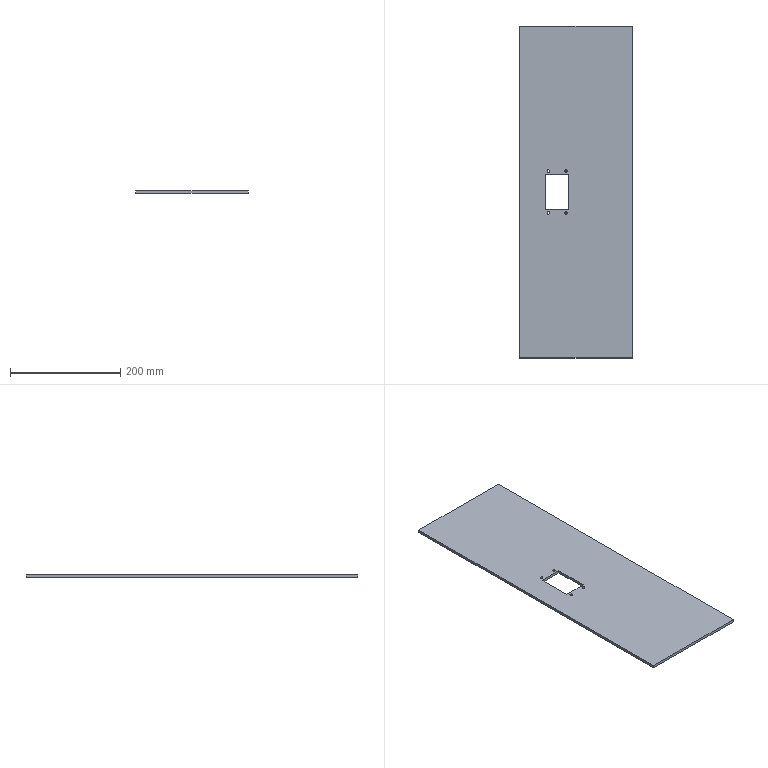Part | NX | features BREP 1 | 1 solid | 18 faces | box 204.5 x 603 x 5 mm | volume 602704 mm3 | plane 10 | cylinder 8 | commonest cylinder face diameters 4.5 x8
STEP:
#1=CARTESIAN_POINT('',(-20.5,-38.,-2.5));
#2=VERTEX_POINT('',#1);
#3=CARTESIAN_POINT('',(-16.,-38.,-2.5));
#4=VERTEX_POINT('',#3);
#5=CARTESIAN_POINT('',(-18.25,-38.,-2.5));
#6=DIRECTION('',(0.,0.,1.));
#7=DIRECTION('',(1.,0.,0.));
#8=AXIS2_PLACEMENT_3D('',#5,#6,#7);
#9=CIRCLE('',#8,2.25);
#10=EDGE_CURVE('',#2,#4,#9,.T.);
#11=ORIENTED_EDGE('',*,*,#10,.F.);
#12=CARTESIAN_POINT('',(-20.5,-38.,2.5));
#13=VERTEX_POINT('',#12);
#14=CARTESIAN_POINT('',(-20.5,-38.,-2.5));
#15=DIRECTION('',(0.,0.,1.));
#16=VECTOR('',#15,1000.);
#17=LINE('',#14,#16);
#18=EDGE_CURVE('',#13,#2,#17,.F.);
#19=ORIENTED_EDGE('',*,*,#18,.F.);
#20=CARTESIAN_POINT('',(-16.,-38.,2.5));
#21=VERTEX_POINT('',#20);
#22=CARTESIAN_POINT('',(-18.25,-38.,2.5));
#23=DIRECTION('',(0.,0.,1.));
#24=DIRECTION('',(1.,0.,0.));
#25=AXIS2_PLACEMENT_3D('',#22,#23,#24);
#26=CIRCLE('',#25,2.25);
#27=EDGE_CURVE('',#13,#21,#26,.T.);
#28=ORIENTED_EDGE('',*,*,#27,.T.);
#29=CARTESIAN_POINT('',(-16.,-38.,-2.5));
#30=DIRECTION('',(0.,0.,1.));
#31=VECTOR('',#30,1000.);
#32=LINE('',#29,#31);
#33=EDGE_CURVE('',#21,#4,#32,.F.);
#34=ORIENTED_EDGE('',*,*,#33,.T.);
#35=EDGE_LOOP('',(#11,#19,#28,#34));
#36=FACE_BOUND('',#35,.T.);
#37=CARTESIAN_POINT('',(-18.25,-38.,-2.5));
#38=DIRECTION('',(0.,0.,1.));
#39=DIRECTION('',(1.,0.,0.));
#40=AXIS2_PLACEMENT_3D('',#37,#38,#39);
#41=CYLINDRICAL_SURFACE('',#40,2.25);
#42=ADVANCED_FACE('',(#36),#41,.F.);
#43=CARTESIAN_POINT('',(-52.5,-38.,-2.5));
#44=VERTEX_POINT('',#43);
#45=CARTESIAN_POINT('',(-48.,-38.,-2.5));
#46=VERTEX_POINT('',#45);
#47=CARTESIAN_POINT('',(-50.25,-38.,-2.5));
#48=DIRECTION('',(0.,0.,1.));
#49=DIRECTION('',(1.,0.,0.));
#50=AXIS2_PLACEMENT_3D('',#47,#48,#49);
#51=CIRCLE('',#50,2.25);
#52=EDGE_CURVE('',#44,#46,#51,.T.);
#53=ORIENTED_EDGE('',*,*,#52,.F.);
#54=CARTESIAN_POINT('',(-52.5,-38.,2.5));
#55=VERTEX_POINT('',#54);
#56=CARTESIAN_POINT('',(-52.5,-38.,-2.5));
#57=DIRECTION('',(0.,0.,1.));
#58=VECTOR('',#57,1000.);
#59=LINE('',#56,#58);
#60=EDGE_CURVE('',#55,#44,#59,.F.);
#61=ORIENTED_EDGE('',*,*,#60,.F.);
#62=CARTESIAN_POINT('',(-48.,-38.,2.5));
#63=VERTEX_POINT('',#62);
#64=CARTESIAN_POINT('',(-50.25,-38.,2.5));
#65=DIRECTION('',(0.,0.,1.));
#66=DIRECTION('',(1.,0.,0.));
#67=AXIS2_PLACEMENT_3D('',#64,#65,#66);
#68=CIRCLE('',#67,2.25);
#69=EDGE_CURVE('',#55,#63,#68,.T.);
#70=ORIENTED_EDGE('',*,*,#69,.T.);
#71=CARTESIAN_POINT('',(-48.,-38.,-2.5));
#72=DIRECTION('',(0.,0.,1.));
#73=VECTOR('',#72,1000.);
#74=LINE('',#71,#73);
#75=EDGE_CURVE('',#63,#46,#74,.F.);
#76=ORIENTED_EDGE('',*,*,#75,.T.);
#77=EDGE_LOOP('',(#53,#61,#70,#76));
#78=FACE_BOUND('',#77,.T.);
#79=CARTESIAN_POINT('',(-50.25,-38.,-2.5));
#80=DIRECTION('',(0.,0.,1.));
#81=DIRECTION('',(1.,0.,0.));
#82=AXIS2_PLACEMENT_3D('',#79,#80,#81);
#83=CYLINDRICAL_SURFACE('',#82,2.25);
#84=ADVANCED_FACE('',(#78),#83,.F.);
#85=CARTESIAN_POINT('',(-20.5,38.,-2.5));
#86=VERTEX_POINT('',#85);
#87=CARTESIAN_POINT('',(-16.,38.,-2.5));
#88=VERTEX_POINT('',#87);
#89=CARTESIAN_POINT('',(-18.25,38.,-2.5));
#90=DIRECTION('',(0.,0.,1.));
#91=DIRECTION('',(1.,0.,0.));
#92=AXIS2_PLACEMENT_3D('',#89,#90,#91);
#93=CIRCLE('',#92,2.25);
#94=EDGE_CURVE('',#86,#88,#93,.T.);
#95=ORIENTED_EDGE('',*,*,#94,.F.);
#96=CARTESIAN_POINT('',(-20.5,38.,2.5));
#97=VERTEX_POINT('',#96);
#98=CARTESIAN_POINT('',(-20.5,38.,-2.5));
#99=DIRECTION('',(0.,0.,1.));
#100=VECTOR('',#99,1000.);
#101=LINE('',#98,#100);
#102=EDGE_CURVE('',#97,#86,#101,.F.);
#103=ORIENTED_EDGE('',*,*,#102,.F.);
#104=CARTESIAN_POINT('',(-16.,38.,2.5));
#105=VERTEX_POINT('',#104);
#106=CARTESIAN_POINT('',(-18.25,38.,2.5));
#107=DIRECTION('',(0.,0.,1.));
#108=DIRECTION('',(1.,0.,0.));
#109=AXIS2_PLACEMENT_3D('',#106,#107,#108);
#110=CIRCLE('',#109,2.25);
#111=EDGE_CURVE('',#97,#105,#110,.T.);
#112=ORIENTED_EDGE('',*,*,#111,.T.);
#113=CARTESIAN_POINT('',(-16.,38.,-2.5));
#114=DIRECTION('',(0.,0.,1.));
#115=VECTOR('',#114,1000.);
#116=LINE('',#113,#115);
#117=EDGE_CURVE('',#105,#88,#116,.F.);
#118=ORIENTED_EDGE('',*,*,#117,.T.);
#119=EDGE_LOOP('',(#95,#103,#112,#118));
#120=FACE_BOUND('',#119,.T.);
#121=CARTESIAN_POINT('',(-18.25,38.,-2.5));
#122=DIRECTION('',(0.,0.,1.));
#123=DIRECTION('',(1.,0.,0.));
#124=AXIS2_PLACEMENT_3D('',#121,#122,#123);
#125=CYLINDRICAL_SURFACE('',#124,2.25);
#126=ADVANCED_FACE('',(#120),#125,.F.);
#127=CARTESIAN_POINT('',(-52.5,38.,-2.5));
#128=VERTEX_POINT('',#127);
#129=CARTESIAN_POINT('',(-48.,38.,-2.5));
#130=VERTEX_POINT('',#129);
#131=CARTESIAN_POINT('',(-50.25,38.,-2.5));
#132=DIRECTION('',(0.,0.,1.));
#133=DIRECTION('',(1.,0.,0.));
#134=AXIS2_PLACEMENT_3D('',#131,#132,#133);
#135=CIRCLE('',#134,2.25);
#136=EDGE_CURVE('',#128,#130,#135,.T.);
#137=ORIENTED_EDGE('',*,*,#136,.F.);
#138=CARTESIAN_POINT('',(-52.5,38.,2.5));
#139=VERTEX_POINT('',#138);
#140=CARTESIAN_POINT('',(-52.5,38.,-2.5));
#141=DIRECTION('',(0.,0.,1.));
#142=VECTOR('',#141,1000.);
#143=LINE('',#140,#142);
#144=EDGE_CURVE('',#139,#128,#143,.F.);
#145=ORIENTED_EDGE('',*,*,#144,.F.);
#146=CARTESIAN_POINT('',(-48.,38.,2.5));
#147=VERTEX_POINT('',#146);
#148=CARTESIAN_POINT('',(-50.25,38.,2.5));
#149=DIRECTION('',(0.,0.,1.));
#150=DIRECTION('',(1.,0.,0.));
#151=AXIS2_PLACEMENT_3D('',#148,#149,#150);
#152=CIRCLE('',#151,2.25);
#153=EDGE_CURVE('',#139,#147,#152,.T.);
#154=ORIENTED_EDGE('',*,*,#153,.T.);
#155=CARTESIAN_POINT('',(-48.,38.,-2.5));
#156=DIRECTION('',(0.,0.,1.));
#157=VECTOR('',#156,1000.);
#158=LINE('',#155,#157);
#159=EDGE_CURVE('',#147,#130,#158,.F.);
#160=ORIENTED_EDGE('',*,*,#159,.T.);
#161=EDGE_LOOP('',(#137,#145,#154,#160));
#162=FACE_BOUND('',#161,.T.);
#163=CARTESIAN_POINT('',(-50.25,38.,-2.5));
#164=DIRECTION('',(0.,0.,1.));
#165=DIRECTION('',(1.,0.,0.));
#166=AXIS2_PLACEMENT_3D('',#163,#164,#165);
#167=CYLINDRICAL_SURFACE('',#166,2.25);
#168=ADVANCED_FACE('',(#162),#167,.F.);
#169=CARTESIAN_POINT('',(102.25,-301.5,-2.5));
#170=VERTEX_POINT('',#169);
#171=CARTESIAN_POINT('',(102.25,301.5,-2.5));
#172=VERTEX_POINT('',#171);
#173=CARTESIAN_POINT('',(102.25,-301.5,-2.5));
#174=DIRECTION('',(0.,1.,0.));
#175=VECTOR('',#174,1000.);
#176=LINE('',#173,#175);
#177=EDGE_CURVE('',#170,#172,#176,.T.);
#178=ORIENTED_EDGE('',*,*,#177,.T.);
#179=CARTESIAN_POINT('',(102.25,301.5,2.5));
#180=VERTEX_POINT('',#179);
#181=CARTESIAN_POINT('',(102.25,301.5,2.5));
#182=DIRECTION('',(0.,0.,-1.));
#183=VECTOR('',#182,1000.);
#184=LINE('',#181,#183);
#185=EDGE_CURVE('',#180,#172,#184,.T.);
#186=ORIENTED_EDGE('',*,*,#185,.F.);
#187=CARTESIAN_POINT('',(102.25,-301.5,2.5));
#188=VERTEX_POINT('',#187);
#189=CARTESIAN_POINT('',(102.25,-301.5,2.5));
#190=DIRECTION('',(0.,1.,0.));
#191=VECTOR('',#190,1000.);
#192=LINE('',#189,#191);
#193=EDGE_CURVE('',#188,#180,#192,.T.);
#194=ORIENTED_EDGE('',*,*,#193,.F.);
#195=CARTESIAN_POINT('',(102.25,-301.5,2.5));
#196=DIRECTION('',(0.,0.,-1.));
#197=VECTOR('',#196,1000.);
#198=LINE('',#195,#197);
#199=EDGE_CURVE('',#188,#170,#198,.T.);
#200=ORIENTED_EDGE('',*,*,#199,.T.);
#201=EDGE_LOOP('',(#178,#186,#194,#200));
#202=FACE_BOUND('',#201,.T.);
#203=CARTESIAN_POINT('',(102.25,-301.5,2.5));
#204=DIRECTION('',(-1.,0.,0.));
#205=DIRECTION('',(0.,0.,1.));
#206=AXIS2_PLACEMENT_3D('',#203,#204,#205);
#207=PLANE('',#206);
#208=ADVANCED_FACE('',(#202),#207,.F.);
#209=CARTESIAN_POINT('',(-102.25,301.5,-2.5));
#210=VERTEX_POINT('',#209);
#211=CARTESIAN_POINT('',(-102.25,301.5,-2.5));
#212=DIRECTION('',(-1.,0.,0.));
#213=VECTOR('',#212,1000.);
#214=LINE('',#211,#213);
#215=EDGE_CURVE('',#172,#210,#214,.T.);
#216=ORIENTED_EDGE('',*,*,#215,.T.);
#217=CARTESIAN_POINT('',(-102.25,301.5,2.5));
#218=VERTEX_POINT('',#217);
#219=CARTESIAN_POINT('',(-102.25,301.5,2.5));
#220=DIRECTION('',(0.,0.,-1.));
#221=VECTOR('',#220,1000.);
#222=LINE('',#219,#221);
#223=EDGE_CURVE('',#218,#210,#222,.T.);
#224=ORIENTED_EDGE('',*,*,#223,.F.);
#225=CARTESIAN_POINT('',(-102.25,301.5,2.5));
#226=DIRECTION('',(-1.,0.,0.));
#227=VECTOR('',#226,1000.);
#228=LINE('',#225,#227);
#229=EDGE_CURVE('',#180,#218,#228,.T.);
#230=ORIENTED_EDGE('',*,*,#229,.F.);
#231=ORIENTED_EDGE('',*,*,#185,.T.);
#232=EDGE_LOOP('',(#216,#224,#230,#231));
#233=FACE_BOUND('',#232,.T.);
#234=CARTESIAN_POINT('',(-102.25,301.5,2.5));
#235=DIRECTION('',(0.,-1.,0.));
#236=DIRECTION('',(0.,0.,-1.));
#237=AXIS2_PLACEMENT_3D('',#234,#235,#236);
#238=PLANE('',#237);
#239=ADVANCED_FACE('',(#233),#238,.F.);
#240=CARTESIAN_POINT('',(-102.25,-301.5,-2.5));
#241=VERTEX_POINT('',#240);
#242=CARTESIAN_POINT('',(-102.25,-301.5,-2.5));
#243=DIRECTION('',(0.,-1.,0.));
#244=VECTOR('',#243,1000.);
#245=LINE('',#242,#244);
#246=EDGE_CURVE('',#210,#241,#245,.T.);
#247=ORIENTED_EDGE('',*,*,#246,.T.);
#248=CARTESIAN_POINT('',(-102.25,-301.5,2.5));
#249=VERTEX_POINT('',#248);
#250=CARTESIAN_POINT('',(-102.25,-301.5,2.5));
#251=DIRECTION('',(0.,0.,-1.));
#252=VECTOR('',#251,1000.);
#253=LINE('',#250,#252);
#254=EDGE_CURVE('',#249,#241,#253,.T.);
#255=ORIENTED_EDGE('',*,*,#254,.F.);
#256=CARTESIAN_POINT('',(-102.25,-301.5,2.5));
#257=DIRECTION('',(0.,-1.,0.));
#258=VECTOR('',#257,1000.);
#259=LINE('',#256,#258);
#260=EDGE_CURVE('',#218,#249,#259,.T.);
#261=ORIENTED_EDGE('',*,*,#260,.F.);
#262=ORIENTED_EDGE('',*,*,#223,.T.);
#263=EDGE_LOOP('',(#247,#255,#261,#262));
#264=FACE_BOUND('',#263,.T.);
#265=CARTESIAN_POINT('',(-102.25,-301.5,2.5));
#266=DIRECTION('',(1.,0.,0.));
#267=DIRECTION('',(0.,1.,0.));
#268=AXIS2_PLACEMENT_3D('',#265,#266,#267);
#269=PLANE('',#268);
#270=ADVANCED_FACE('',(#264),#269,.F.);
#271=CARTESIAN_POINT('',(-102.25,-301.5,-2.5));
#272=DIRECTION('',(1.,0.,0.));
#273=VECTOR('',#272,1000.);
#274=LINE('',#271,#273);
#275=EDGE_CURVE('',#241,#170,#274,.T.);
#276=ORIENTED_EDGE('',*,*,#275,.T.);
#277=ORIENTED_EDGE('',*,*,#199,.F.);
#278=CARTESIAN_POINT('',(-102.25,-301.5,2.5));
#279=DIRECTION('',(1.,0.,0.));
#280=VECTOR('',#279,1000.);
#281=LINE('',#278,#280);
#282=EDGE_CURVE('',#249,#188,#281,.T.);
#283=ORIENTED_EDGE('',*,*,#282,.F.);
#284=ORIENTED_EDGE('',*,*,#254,.T.);
#285=EDGE_LOOP('',(#276,#277,#283,#284));
#286=FACE_BOUND('',#285,.T.);
#287=CARTESIAN_POINT('',(-102.25,-301.5,2.5));
#288=DIRECTION('',(0.,1.,0.));
#289=DIRECTION('',(1.,0.,0.));
#290=AXIS2_PLACEMENT_3D('',#287,#288,#289);
#291=PLANE('',#290);
#292=ADVANCED_FACE('',(#286),#291,.F.);
#293=ORIENTED_EDGE('',*,*,#193,.T.);
#294=ORIENTED_EDGE('',*,*,#229,.T.);
#295=ORIENTED_EDGE('',*,*,#260,.T.);
#296=ORIENTED_EDGE('',*,*,#282,.T.);
#297=EDGE_LOOP('',(#293,#294,#295,#296));
#298=FACE_BOUND('',#297,.T.);
#299=CARTESIAN_POINT('',(-18.25,-38.,2.5));
#300=DIRECTION('',(0.,0.,1.));
#301=DIRECTION('',(1.,0.,0.));
#302=AXIS2_PLACEMENT_3D('',#299,#300,#301);
#303=CIRCLE('',#302,2.25);
#304=EDGE_CURVE('',#21,#13,#303,.T.);
#305=ORIENTED_EDGE('',*,*,#304,.F.);
#306=ORIENTED_EDGE('',*,*,#27,.F.);
#307=EDGE_LOOP('',(#305,#306));
#308=FACE_BOUND('',#307,.T.);
#309=CARTESIAN_POINT('',(-50.25,-38.,2.5));
#310=DIRECTION('',(0.,0.,1.));
#311=DIRECTION('',(1.,0.,0.));
#312=AXIS2_PLACEMENT_3D('',#309,#310,#311);
#313=CIRCLE('',#312,2.25);
#314=EDGE_CURVE('',#63,#55,#313,.T.);
#315=ORIENTED_EDGE('',*,*,#314,.F.);
#316=ORIENTED_EDGE('',*,*,#69,.F.);
#317=EDGE_LOOP('',(#315,#316));
#318=FACE_BOUND('',#317,.T.);
#319=CARTESIAN_POINT('',(-18.25,38.,2.5));
#320=DIRECTION('',(0.,0.,1.));
#321=DIRECTION('',(1.,0.,0.));
#322=AXIS2_PLACEMENT_3D('',#319,#320,#321);
#323=CIRCLE('',#322,2.25);
#324=EDGE_CURVE('',#105,#97,#323,.T.);
#325=ORIENTED_EDGE('',*,*,#324,.F.);
#326=ORIENTED_EDGE('',*,*,#111,.F.);
#327=EDGE_LOOP('',(#325,#326));
#328=FACE_BOUND('',#327,.T.);
#329=CARTESIAN_POINT('',(-50.25,38.,2.5));
#330=DIRECTION('',(0.,0.,1.));
#331=DIRECTION('',(1.,0.,0.));
#332=AXIS2_PLACEMENT_3D('',#329,#330,#331);
#333=CIRCLE('',#332,2.25);
#334=EDGE_CURVE('',#147,#139,#333,.T.);
#335=ORIENTED_EDGE('',*,*,#334,.F.);
#336=ORIENTED_EDGE('',*,*,#153,.F.);
#337=EDGE_LOOP('',(#335,#336));
#338=FACE_BOUND('',#337,.T.);
#339=CARTESIAN_POINT('',(-12.75,31.5,2.5));
#340=VERTEX_POINT('',#339);
#341=CARTESIAN_POINT('',(-55.75,31.5,2.5));
#342=VERTEX_POINT('',#341);
#343=CARTESIAN_POINT('',(-55.75,31.5,2.5));
#344=DIRECTION('',(-1.,0.,0.));
#345=VECTOR('',#344,1000.);
#346=LINE('',#343,#345);
#347=EDGE_CURVE('',#340,#342,#346,.T.);
#348=ORIENTED_EDGE('',*,*,#347,.F.);
#349=CARTESIAN_POINT('',(-12.75,-31.5,2.5));
#350=VERTEX_POINT('',#349);
#351=CARTESIAN_POINT('',(-12.75,-31.5,2.5));
#352=DIRECTION('',(0.,1.,0.));
#353=VECTOR('',#352,1000.);
#354=LINE('',#351,#353);
#355=EDGE_CURVE('',#350,#340,#354,.T.);
#356=ORIENTED_EDGE('',*,*,#355,.F.);
#357=CARTESIAN_POINT('',(-55.75,-31.5,2.5));
#358=VERTEX_POINT('',#357);
#359=CARTESIAN_POINT('',(-55.75,-31.5,2.5));
#360=DIRECTION('',(1.,0.,0.));
#361=VECTOR('',#360,1000.);
#362=LINE('',#359,#361);
#363=EDGE_CURVE('',#358,#350,#362,.T.);
#364=ORIENTED_EDGE('',*,*,#363,.F.);
#365=CARTESIAN_POINT('',(-55.75,-31.5,2.5));
#366=DIRECTION('',(0.,-1.,0.));
#367=VECTOR('',#366,1000.);
#368=LINE('',#365,#367);
#369=EDGE_CURVE('',#342,#358,#368,.T.);
#370=ORIENTED_EDGE('',*,*,#369,.F.);
#371=EDGE_LOOP('',(#348,#356,#364,#370));
#372=FACE_BOUND('',#371,.T.);
#373=CARTESIAN_POINT('',(0.,0.,2.5));
#374=DIRECTION('',(0.,0.,-1.));
#375=DIRECTION('',(0.,-1.,0.));
#376=AXIS2_PLACEMENT_3D('',#373,#374,#375);
#377=PLANE('',#376);
#378=ADVANCED_FACE('',(#298,#308,#318,#328,#338,#372),#377,.F.);
#379=ORIENTED_EDGE('',*,*,#177,.F.);
#380=ORIENTED_EDGE('',*,*,#275,.F.);
#381=ORIENTED_EDGE('',*,*,#246,.F.);
#382=ORIENTED_EDGE('',*,*,#215,.F.);
#383=EDGE_LOOP('',(#379,#380,#381,#382));
#384=FACE_BOUND('',#383,.T.);
#385=CARTESIAN_POINT('',(-18.25,-38.,-2.5));
#386=DIRECTION('',(0.,0.,1.));
#387=DIRECTION('',(1.,0.,0.));
#388=AXIS2_PLACEMENT_3D('',#385,#386,#387);
#389=CIRCLE('',#388,2.25);
#390=EDGE_CURVE('',#4,#2,#389,.T.);
#391=ORIENTED_EDGE('',*,*,#390,.T.);
#392=ORIENTED_EDGE('',*,*,#10,.T.);
#393=EDGE_LOOP('',(#391,#392));
#394=FACE_BOUND('',#393,.T.);
#395=CARTESIAN_POINT('',(-50.25,-38.,-2.5));
#396=DIRECTION('',(0.,0.,1.));
#397=DIRECTION('',(1.,0.,0.));
#398=AXIS2_PLACEMENT_3D('',#395,#396,#397);
#399=CIRCLE('',#398,2.25);
#400=EDGE_CURVE('',#46,#44,#399,.T.);
#401=ORIENTED_EDGE('',*,*,#400,.T.);
#402=ORIENTED_EDGE('',*,*,#52,.T.);
#403=EDGE_LOOP('',(#401,#402));
#404=FACE_BOUND('',#403,.T.);
#405=CARTESIAN_POINT('',(-18.25,38.,-2.5));
#406=DIRECTION('',(0.,0.,1.));
#407=DIRECTION('',(1.,0.,0.));
#408=AXIS2_PLACEMENT_3D('',#405,#406,#407);
#409=CIRCLE('',#408,2.25);
#410=EDGE_CURVE('',#88,#86,#409,.T.);
#411=ORIENTED_EDGE('',*,*,#410,.T.);
#412=ORIENTED_EDGE('',*,*,#94,.T.);
#413=EDGE_LOOP('',(#411,#412));
#414=FACE_BOUND('',#413,.T.);
#415=CARTESIAN_POINT('',(-50.25,38.,-2.5));
#416=DIRECTION('',(0.,0.,1.));
#417=DIRECTION('',(1.,0.,0.));
#418=AXIS2_PLACEMENT_3D('',#415,#416,#417);
#419=CIRCLE('',#418,2.25);
#420=EDGE_CURVE('',#130,#128,#419,.T.);
#421=ORIENTED_EDGE('',*,*,#420,.T.);
#422=ORIENTED_EDGE('',*,*,#136,.T.);
#423=EDGE_LOOP('',(#421,#422));
#424=FACE_BOUND('',#423,.T.);
#425=CARTESIAN_POINT('',(-12.75,-31.5,-2.5));
#426=VERTEX_POINT('',#425);
#427=CARTESIAN_POINT('',(-12.75,31.5,-2.5));
#428=VERTEX_POINT('',#427);
#429=CARTESIAN_POINT('',(-12.75,-31.5,-2.5));
#430=DIRECTION('',(0.,1.,0.));
#431=VECTOR('',#430,1000.);
#432=LINE('',#429,#431);
#433=EDGE_CURVE('',#426,#428,#432,.T.);
#434=ORIENTED_EDGE('',*,*,#433,.T.);
#435=CARTESIAN_POINT('',(-55.75,31.5,-2.5));
#436=VERTEX_POINT('',#435);
#437=CARTESIAN_POINT('',(-55.75,31.5,-2.5));
#438=DIRECTION('',(-1.,0.,0.));
#439=VECTOR('',#438,1000.);
#440=LINE('',#437,#439);
#441=EDGE_CURVE('',#428,#436,#440,.T.);
#442=ORIENTED_EDGE('',*,*,#441,.T.);
#443=CARTESIAN_POINT('',(-55.75,-31.5,-2.5));
#444=VERTEX_POINT('',#443);
#445=CARTESIAN_POINT('',(-55.75,-31.5,-2.5));
#446=DIRECTION('',(0.,-1.,0.));
#447=VECTOR('',#446,1000.);
#448=LINE('',#445,#447);
#449=EDGE_CURVE('',#436,#444,#448,.T.);
#450=ORIENTED_EDGE('',*,*,#449,.T.);
#451=CARTESIAN_POINT('',(-55.75,-31.5,-2.5));
#452=DIRECTION('',(1.,0.,0.));
#453=VECTOR('',#452,1000.);
#454=LINE('',#451,#453);
#455=EDGE_CURVE('',#444,#426,#454,.T.);
#456=ORIENTED_EDGE('',*,*,#455,.T.);
#457=EDGE_LOOP('',(#434,#442,#450,#456));
#458=FACE_BOUND('',#457,.T.);
#459=CARTESIAN_POINT('',(0.,0.,-2.5));
#460=DIRECTION('',(0.,0.,-1.));
#461=DIRECTION('',(0.,-1.,0.));
#462=AXIS2_PLACEMENT_3D('',#459,#460,#461);
#463=PLANE('',#462);
#464=ADVANCED_FACE('',(#384,#394,#404,#414,#424,#458),#463,.T.);
#465=CARTESIAN_POINT('',(-12.75,31.5,-2.5));
#466=DIRECTION('',(0.,0.,1.));
#467=VECTOR('',#466,1000.);
#468=LINE('',#465,#467);
#469=EDGE_CURVE('',#428,#340,#468,.T.);
#470=ORIENTED_EDGE('',*,*,#469,.F.);
#471=ORIENTED_EDGE('',*,*,#433,.F.);
#472=CARTESIAN_POINT('',(-12.75,-31.5,-2.5));
#473=DIRECTION('',(0.,0.,1.));
#474=VECTOR('',#473,1000.);
#475=LINE('',#472,#474);
#476=EDGE_CURVE('',#426,#350,#475,.T.);
#477=ORIENTED_EDGE('',*,*,#476,.T.);
#478=ORIENTED_EDGE('',*,*,#355,.T.);
#479=EDGE_LOOP('',(#470,#471,#477,#478));
#480=FACE_BOUND('',#479,.T.);
#481=CARTESIAN_POINT('',(-12.75,-31.5,-2.5));
#482=DIRECTION('',(1.,0.,0.));
#483=DIRECTION('',(0.,1.,0.));
#484=AXIS2_PLACEMENT_3D('',#481,#482,#483);
#485=PLANE('',#484);
#486=ADVANCED_FACE('',(#480),#485,.F.);
#487=ORIENTED_EDGE('',*,*,#476,.F.);
#488=ORIENTED_EDGE('',*,*,#455,.F.);
#489=CARTESIAN_POINT('',(-55.75,-31.5,-2.5));
#490=DIRECTION('',(0.,0.,1.));
#491=VECTOR('',#490,1000.);
#492=LINE('',#489,#491);
#493=EDGE_CURVE('',#444,#358,#492,.T.);
#494=ORIENTED_EDGE('',*,*,#493,.T.);
#495=ORIENTED_EDGE('',*,*,#363,.T.);
#496=EDGE_LOOP('',(#487,#488,#494,#495));
#497=FACE_BOUND('',#496,.T.);
#498=CARTESIAN_POINT('',(-55.75,-31.5,-2.5));
#499=DIRECTION('',(0.,-1.,0.));
#500=DIRECTION('',(0.,0.,-1.));
#501=AXIS2_PLACEMENT_3D('',#498,#499,#500);
#502=PLANE('',#501);
#503=ADVANCED_FACE('',(#497),#502,.F.);
#504=ORIENTED_EDGE('',*,*,#493,.F.);
#505=ORIENTED_EDGE('',*,*,#449,.F.);
#506=CARTESIAN_POINT('',(-55.75,31.5,-2.5));
#507=DIRECTION('',(0.,0.,1.));
#508=VECTOR('',#507,1000.);
#509=LINE('',#506,#508);
#510=EDGE_CURVE('',#436,#342,#509,.T.);
#511=ORIENTED_EDGE('',*,*,#510,.T.);
#512=ORIENTED_EDGE('',*,*,#369,.T.);
#513=EDGE_LOOP('',(#504,#505,#511,#512));
#514=FACE_BOUND('',#513,.T.);
#515=CARTESIAN_POINT('',(-55.75,-31.5,-2.5));
#516=DIRECTION('',(-1.,0.,0.));
#517=DIRECTION('',(0.,0.,1.));
#518=AXIS2_PLACEMENT_3D('',#515,#516,#517);
#519=PLANE('',#518);
#520=ADVANCED_FACE('',(#514),#519,.F.);
#521=ORIENTED_EDGE('',*,*,#510,.F.);
#522=ORIENTED_EDGE('',*,*,#441,.F.);
#523=ORIENTED_EDGE('',*,*,#469,.T.);
#524=ORIENTED_EDGE('',*,*,#347,.T.);
#525=EDGE_LOOP('',(#521,#522,#523,#524));
#526=FACE_BOUND('',#525,.T.);
#527=CARTESIAN_POINT('',(-55.75,31.5,-2.5));
#528=DIRECTION('',(0.,1.,0.));
#529=DIRECTION('',(1.,0.,0.));
#530=AXIS2_PLACEMENT_3D('',#527,#528,#529);
#531=PLANE('',#530);
#532=ADVANCED_FACE('',(#526),#531,.F.);
#533=ORIENTED_EDGE('',*,*,#144,.T.);
#534=ORIENTED_EDGE('',*,*,#420,.F.);
#535=ORIENTED_EDGE('',*,*,#159,.F.);
#536=ORIENTED_EDGE('',*,*,#334,.T.);
#537=EDGE_LOOP('',(#533,#534,#535,#536));
#538=FACE_BOUND('',#537,.T.);
#539=CARTESIAN_POINT('',(-50.25,38.,-2.5));
#540=DIRECTION('',(0.,0.,1.));
#541=DIRECTION('',(1.,0.,0.));
#542=AXIS2_PLACEMENT_3D('',#539,#540,#541);
#543=CYLINDRICAL_SURFACE('',#542,2.25);
#544=ADVANCED_FACE('',(#538),#543,.F.);
#545=ORIENTED_EDGE('',*,*,#102,.T.);
#546=ORIENTED_EDGE('',*,*,#410,.F.);
#547=ORIENTED_EDGE('',*,*,#117,.F.);
#548=ORIENTED_EDGE('',*,*,#324,.T.);
#549=EDGE_LOOP('',(#545,#546,#547,#548));
#550=FACE_BOUND('',#549,.T.);
#551=CARTESIAN_POINT('',(-18.25,38.,-2.5));
#552=DIRECTION('',(0.,0.,1.));
#553=DIRECTION('',(1.,0.,0.));
#554=AXIS2_PLACEMENT_3D('',#551,#552,#553);
#555=CYLINDRICAL_SURFACE('',#554,2.25);
#556=ADVANCED_FACE('',(#550),#555,.F.);
#557=ORIENTED_EDGE('',*,*,#60,.T.);
#558=ORIENTED_EDGE('',*,*,#400,.F.);
#559=ORIENTED_EDGE('',*,*,#75,.F.);
#560=ORIENTED_EDGE('',*,*,#314,.T.);
#561=EDGE_LOOP('',(#557,#558,#559,#560));
#562=FACE_BOUND('',#561,.T.);
#563=CARTESIAN_POINT('',(-50.25,-38.,-2.5));
#564=DIRECTION('',(0.,0.,1.));
#565=DIRECTION('',(1.,0.,0.));
#566=AXIS2_PLACEMENT_3D('',#563,#564,#565);
#567=CYLINDRICAL_SURFACE('',#566,2.25);
#568=ADVANCED_FACE('',(#562),#567,.F.);
#569=ORIENTED_EDGE('',*,*,#18,.T.);
#570=ORIENTED_EDGE('',*,*,#390,.F.);
#571=ORIENTED_EDGE('',*,*,#33,.F.);
#572=ORIENTED_EDGE('',*,*,#304,.T.);
#573=EDGE_LOOP('',(#569,#570,#571,#572));
#574=FACE_BOUND('',#573,.T.);
#575=CARTESIAN_POINT('',(-18.25,-38.,-2.5));
#576=DIRECTION('',(0.,0.,1.));
#577=DIRECTION('',(1.,0.,0.));
#578=AXIS2_PLACEMENT_3D('',#575,#576,#577);
#579=CYLINDRICAL_SURFACE('',#578,2.25);
#580=ADVANCED_FACE('',(#574),#579,.F.);
#581=CLOSED_SHELL('',(#42,#84,#126,#168,#208,#239,#270,#292,#378,#464,#486,#503,#520,#532,#544,#556,#568,#580));
#582=MANIFOLD_SOLID_BREP('',#581);
#583=(LENGTH_UNIT()NAMED_UNIT(*)SI_UNIT(.MILLI.,.METRE.));
#584=UNCERTAINTY_MEASURE_WITH_UNIT(LENGTH_MEASURE(0.00001),#583,'','');
#585=(NAMED_UNIT(*)PLANE_ANGLE_UNIT()SI_UNIT($,.RADIAN.));
#586=(NAMED_UNIT(*)SI_UNIT($,.STERADIAN.)SOLID_ANGLE_UNIT());
#587=(GEOMETRIC_REPRESENTATION_CONTEXT(3)GLOBAL_UNCERTAINTY_ASSIGNED_CONTEXT((#584))GLOBAL_UNIT_ASSIGNED_CONTEXT((#583,#585,#586))REPRESENTATION_CONTEXT('',''));
#588=ADVANCED_BREP_SHAPE_REPRESENTATION('',(#582),#587);